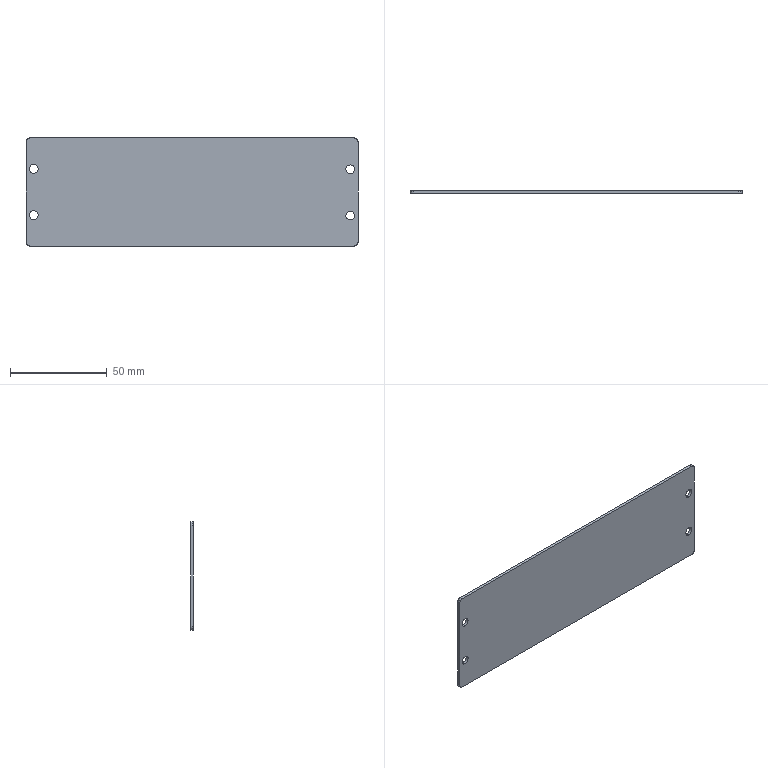Part | STEP file | ASND-0110-TCTF01-30(default)-2 | 1 solid | 22 faces | box 172 x 1.5 x 56 mm | volume 14347 mm3 | cylinder 16 | plane 6 | commonest cylinder face diameters 4 x8 4.5 x8